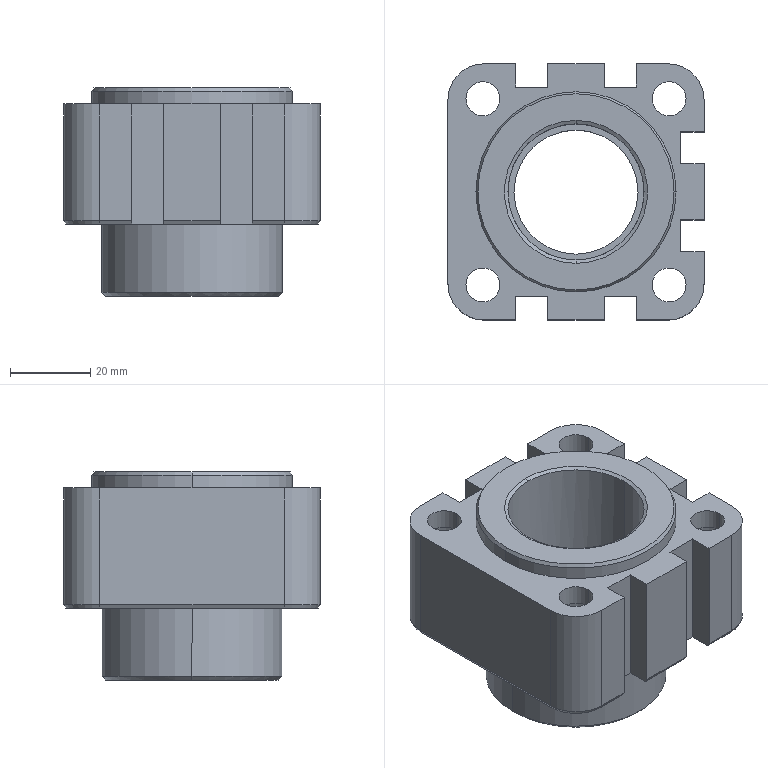Part | SolidWorks | features BaseBody 1 | 1 solid | 99 faces | box 64 x 64 x 52 mm | volume 89017 mm3 | plane 49 | cylinder 32 | cone 18 | commonest cylinder face diameters 8.5 x8 12.5 x8 18 x4 34 x4 31 x2 38 x2